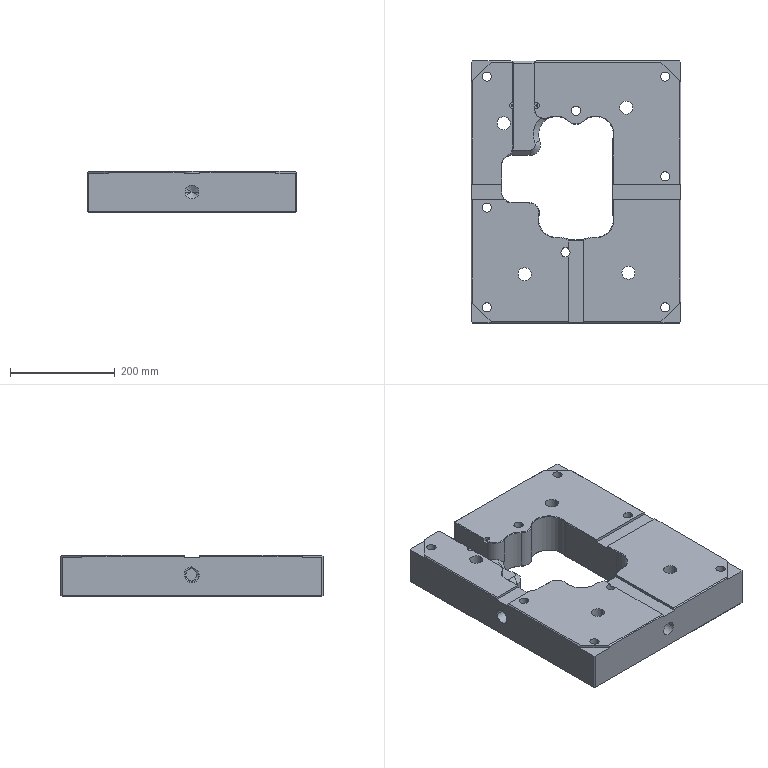Part | Creo | 1 solid | 359 faces | box 400 x 500 x 80 mm | volume 12137396 mm3 | plane 135 | other 101 | cylinder 72 | cone 51 | commonest cylinder face diameters 17.5 x16 40 x11 5 x8 25 x8 10 x6 68 x6